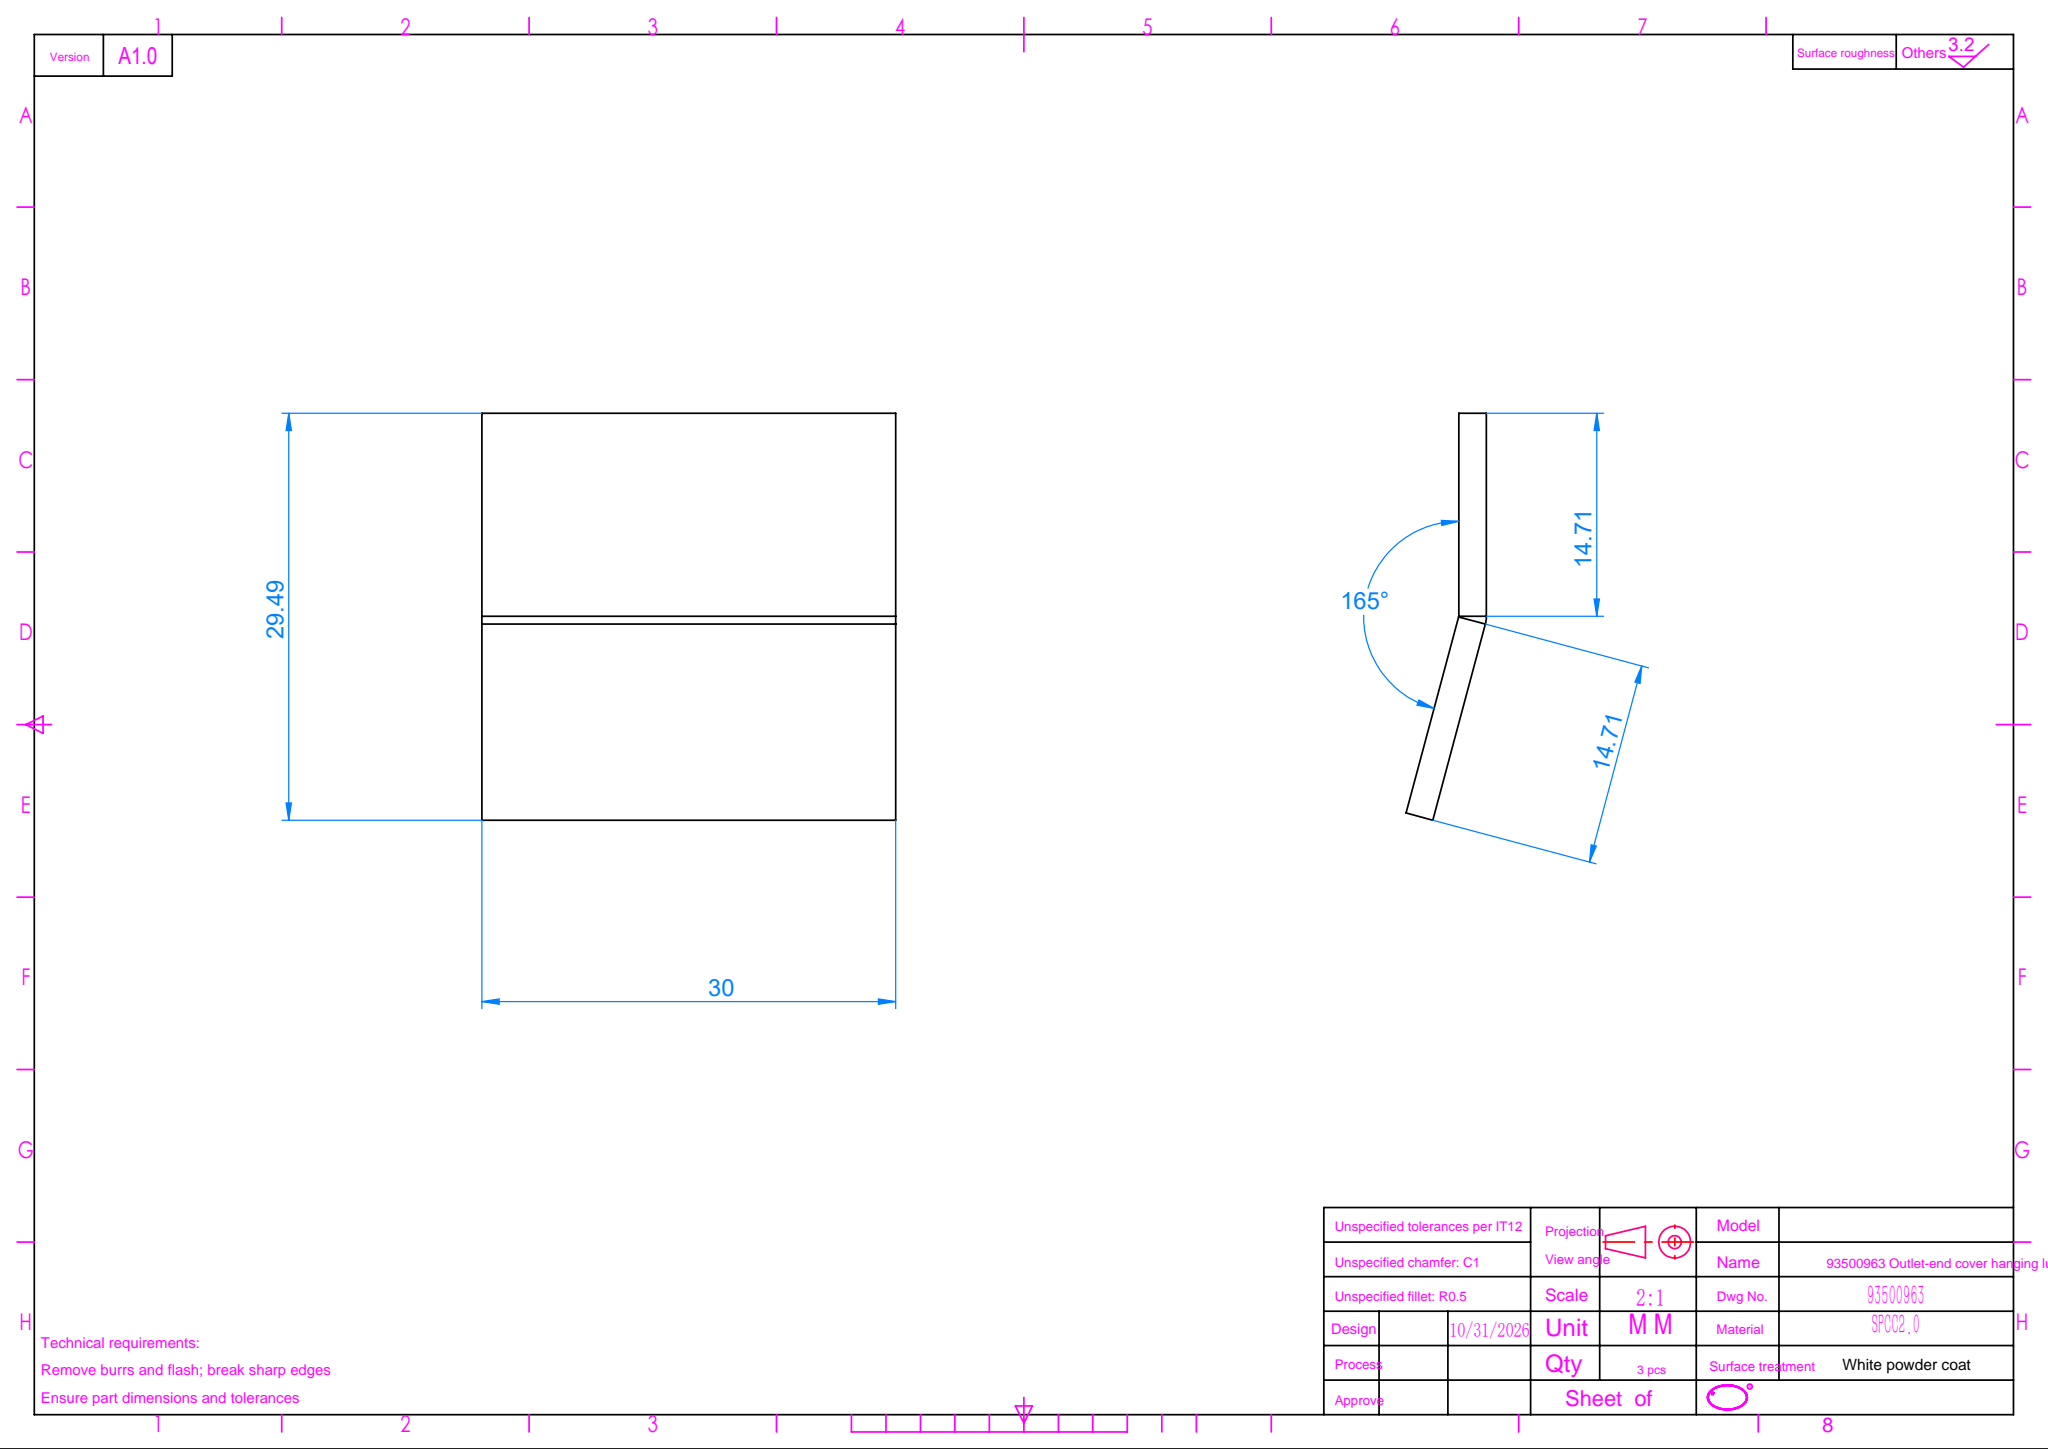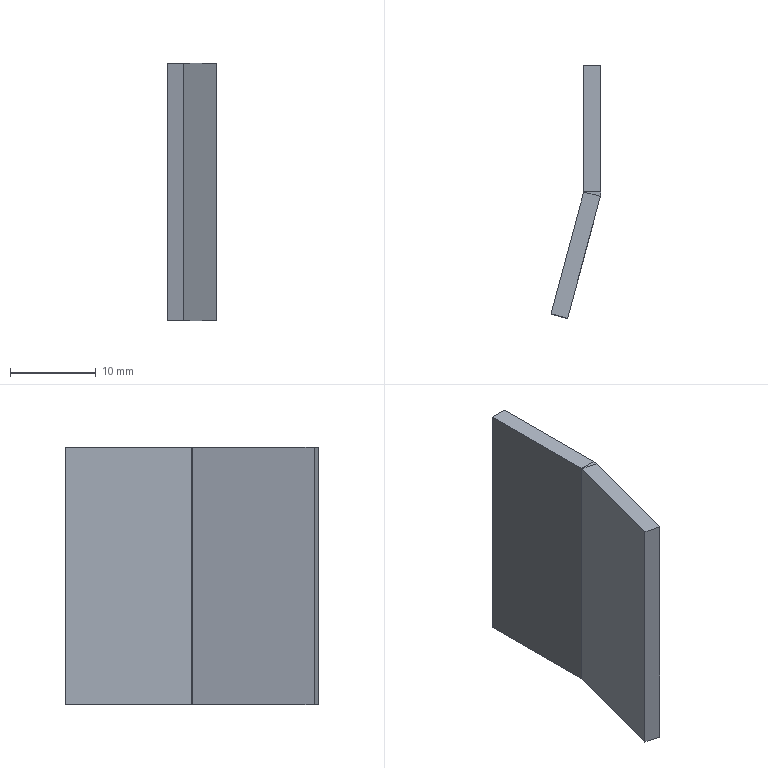Part | SolidWorks | features FlatPattern 1, SMBaseFlange 1, SheetMetal 1 | 1 solid | 14 faces | box 5.814 x 29.489 x 30 mm | volume 1784 mm3 | plane 12 | cylinder 2 | commonest cylinder face diameters 0.4 x1 4.4 x1
STEP:
#1=CARTESIAN_POINT('',(-7.902,11.304,15.));
#2=VERTEX_POINT('',#1);
#3=CARTESIAN_POINT('',(-9.834,11.822,15.));
#4=VERTEX_POINT('',#3);
#5=CARTESIAN_POINT('',(-7.902,11.304,15.));
#6=DIRECTION('',(-0.9659,0.2588,0.));
#7=VECTOR('',#6,1000.);
#8=LINE('',#5,#7);
#9=EDGE_CURVE('',#2,#4,#8,.T.);
#10=ORIENTED_EDGE('',*,*,#9,.F.);
#11=CARTESIAN_POINT('',(-7.827,11.874,15.));
#12=VERTEX_POINT('',#11);
#13=CARTESIAN_POINT('',(-10.027,11.874,15.));
#14=DIRECTION('',(0.,0.,-1.));
#15=DIRECTION('',(1.,0.,0.));
#16=AXIS2_PLACEMENT_3D('',#13,#14,#15);
#17=CIRCLE('',#16,2.2);
#18=EDGE_CURVE('',#12,#2,#17,.T.);
#19=ORIENTED_EDGE('',*,*,#18,.F.);
#20=CARTESIAN_POINT('',(-9.827,11.874,15.));
#21=VERTEX_POINT('',#20);
#22=CARTESIAN_POINT('',(-9.827,11.874,15.));
#23=DIRECTION('',(1.,0.,0.));
#24=VECTOR('',#23,1000.);
#25=LINE('',#22,#24);
#26=EDGE_CURVE('',#21,#12,#25,.T.);
#27=ORIENTED_EDGE('',*,*,#26,.F.);
#28=CARTESIAN_POINT('',(-10.027,11.874,15.));
#29=DIRECTION('',(0.,0.,-1.));
#30=DIRECTION('',(1.,0.,0.));
#31=AXIS2_PLACEMENT_3D('',#28,#29,#30);
#32=CIRCLE('',#31,0.2);
#33=EDGE_CURVE('',#21,#4,#32,.T.);
#34=ORIENTED_EDGE('',*,*,#33,.T.);
#35=EDGE_LOOP('',(#10,#19,#27,#34));
#36=FACE_OUTER_BOUND('',#35,.T.);
#37=CARTESIAN_POINT('',(-7.902,11.304,15.));
#38=DIRECTION('',(0.,0.,1.));
#39=DIRECTION('',(1.,0.,0.));
#40=AXIS2_PLACEMENT_3D('',#37,#38,#39);
#41=PLANE('',#40);
#42=ADVANCED_FACE('',(#36),#41,.T.);
#43=CARTESIAN_POINT('',(-11.71,-2.905,15.));
#44=VERTEX_POINT('',#43);
#45=CARTESIAN_POINT('',(-7.827,11.584,15.));
#46=DIRECTION('',(-0.2588,-0.9659,0.));
#47=VECTOR('',#46,1000.);
#48=LINE('',#45,#47);
#49=EDGE_CURVE('',#2,#44,#48,.T.);
#50=ORIENTED_EDGE('',*,*,#49,.F.);
#51=ORIENTED_EDGE('',*,*,#9,.T.);
#52=CARTESIAN_POINT('',(-13.642,-2.387,15.));
#53=VERTEX_POINT('',#52);
#54=CARTESIAN_POINT('',(-9.759,12.102,15.));
#55=DIRECTION('',(-0.2588,-0.9659,0.));
#56=VECTOR('',#55,1000.);
#57=LINE('',#54,#56);
#58=EDGE_CURVE('',#4,#53,#57,.T.);
#59=ORIENTED_EDGE('',*,*,#58,.T.);
#60=CARTESIAN_POINT('',(-11.71,-2.905,15.));
#61=DIRECTION('',(-0.9659,0.2588,0.));
#62=VECTOR('',#61,1000.);
#63=LINE('',#60,#62);
#64=EDGE_CURVE('',#44,#53,#63,.T.);
#65=ORIENTED_EDGE('',*,*,#64,.F.);
#66=EDGE_LOOP('',(#50,#51,#59,#65));
#67=FACE_OUTER_BOUND('',#66,.T.);
#68=CARTESIAN_POINT('',(-9.827,11.874,15.));
#69=DIRECTION('',(0.,0.,1.));
#70=DIRECTION('',(1.,0.,0.));
#71=AXIS2_PLACEMENT_3D('',#68,#69,#70);
#72=PLANE('',#71);
#73=ADVANCED_FACE('',(#67),#72,.T.);
#74=CARTESIAN_POINT('',(-7.827,11.874,-15.));
#75=VERTEX_POINT('',#74);
#76=CARTESIAN_POINT('',(-9.827,11.874,-15.));
#77=VERTEX_POINT('',#76);
#78=CARTESIAN_POINT('',(-7.827,11.874,-15.));
#79=DIRECTION('',(-1.,0.,0.));
#80=VECTOR('',#79,1000.);
#81=LINE('',#78,#80);
#82=EDGE_CURVE('',#75,#77,#81,.T.);
#83=ORIENTED_EDGE('',*,*,#82,.F.);
#84=CARTESIAN_POINT('',(-7.902,11.304,-15.));
#85=VERTEX_POINT('',#84);
#86=CARTESIAN_POINT('',(-10.027,11.874,-15.));
#87=DIRECTION('',(0.,0.,-1.));
#88=DIRECTION('',(1.,0.,0.));
#89=AXIS2_PLACEMENT_3D('',#86,#87,#88);
#90=CIRCLE('',#89,2.2);
#91=EDGE_CURVE('',#75,#85,#90,.T.);
#92=ORIENTED_EDGE('',*,*,#91,.T.);
#93=CARTESIAN_POINT('',(-9.834,11.822,-15.));
#94=VERTEX_POINT('',#93);
#95=CARTESIAN_POINT('',(-9.834,11.822,-15.));
#96=DIRECTION('',(0.9659,-0.2588,0.));
#97=VECTOR('',#96,1000.);
#98=LINE('',#95,#97);
#99=EDGE_CURVE('',#94,#85,#98,.T.);
#100=ORIENTED_EDGE('',*,*,#99,.F.);
#101=CARTESIAN_POINT('',(-10.027,11.874,-15.));
#102=DIRECTION('',(0.,0.,-1.));
#103=DIRECTION('',(1.,0.,0.));
#104=AXIS2_PLACEMENT_3D('',#101,#102,#103);
#105=CIRCLE('',#104,0.2);
#106=EDGE_CURVE('',#77,#94,#105,.T.);
#107=ORIENTED_EDGE('',*,*,#106,.F.);
#108=EDGE_LOOP('',(#83,#92,#100,#107));
#109=FACE_OUTER_BOUND('',#108,.T.);
#110=CARTESIAN_POINT('',(-7.827,11.874,-15.));
#111=DIRECTION('',(0.,0.,-1.));
#112=DIRECTION('',(-1.,0.,0.));
#113=AXIS2_PLACEMENT_3D('',#110,#111,#112);
#114=PLANE('',#113);
#115=ADVANCED_FACE('',(#109),#114,.T.);
#116=CARTESIAN_POINT('',(-7.827,26.584,-15.));
#117=VERTEX_POINT('',#116);
#118=CARTESIAN_POINT('',(-7.827,26.584,-15.));
#119=DIRECTION('',(0.,-1.,0.));
#120=VECTOR('',#119,1000.);
#121=LINE('',#118,#120);
#122=EDGE_CURVE('',#117,#75,#121,.T.);
#123=ORIENTED_EDGE('',*,*,#122,.T.);
#124=ORIENTED_EDGE('',*,*,#82,.T.);
#125=CARTESIAN_POINT('',(-9.827,26.584,-15.));
#126=VERTEX_POINT('',#125);
#127=CARTESIAN_POINT('',(-9.827,26.584,-15.));
#128=DIRECTION('',(0.,-1.,0.));
#129=VECTOR('',#128,1000.);
#130=LINE('',#127,#129);
#131=EDGE_CURVE('',#126,#77,#130,.T.);
#132=ORIENTED_EDGE('',*,*,#131,.F.);
#133=CARTESIAN_POINT('',(-9.827,26.584,-15.));
#134=DIRECTION('',(1.,0.,0.));
#135=VECTOR('',#134,1000.);
#136=LINE('',#133,#135);
#137=EDGE_CURVE('',#126,#117,#136,.T.);
#138=ORIENTED_EDGE('',*,*,#137,.T.);
#139=EDGE_LOOP('',(#123,#124,#132,#138));
#140=FACE_OUTER_BOUND('',#139,.T.);
#141=CARTESIAN_POINT('',(-9.834,11.822,-15.));
#142=DIRECTION('',(0.,0.,-1.));
#143=DIRECTION('',(-1.,0.,0.));
#144=AXIS2_PLACEMENT_3D('',#141,#142,#143);
#145=PLANE('',#144);
#146=ADVANCED_FACE('',(#140),#145,.T.);
#147=CARTESIAN_POINT('',(-9.834,11.822,15.));
#148=DIRECTION('',(0.,0.,-1.));
#149=VECTOR('',#148,1000.);
#150=LINE('',#147,#149);
#151=EDGE_CURVE('',#4,#94,#150,.T.);
#152=ORIENTED_EDGE('',*,*,#151,.T.);
#153=CARTESIAN_POINT('',(-13.642,-2.387,-15.));
#154=VERTEX_POINT('',#153);
#155=CARTESIAN_POINT('',(-9.759,12.102,-15.));
#156=DIRECTION('',(-0.2588,-0.9659,0.));
#157=VECTOR('',#156,1000.);
#158=LINE('',#155,#157);
#159=EDGE_CURVE('',#94,#154,#158,.T.);
#160=ORIENTED_EDGE('',*,*,#159,.T.);
#161=CARTESIAN_POINT('',(-13.642,-2.387,15.));
#162=DIRECTION('',(0.,0.,-1.));
#163=VECTOR('',#162,1000.);
#164=LINE('',#161,#163);
#165=EDGE_CURVE('',#53,#154,#164,.T.);
#166=ORIENTED_EDGE('',*,*,#165,.F.);
#167=ORIENTED_EDGE('',*,*,#58,.F.);
#168=EDGE_LOOP('',(#152,#160,#166,#167));
#169=FACE_OUTER_BOUND('',#168,.T.);
#170=CARTESIAN_POINT('',(-9.759,12.102,15.));
#171=DIRECTION('',(0.9659,-0.2588,0.));
#172=DIRECTION('',(0.2588,0.9659,0.));
#173=AXIS2_PLACEMENT_3D('',#170,#171,#172);
#174=PLANE('',#173);
#175=ADVANCED_FACE('',(#169),#174,.F.);
#176=ORIENTED_EDGE('',*,*,#165,.T.);
#177=CARTESIAN_POINT('',(-11.71,-2.905,-15.));
#178=VERTEX_POINT('',#177);
#179=CARTESIAN_POINT('',(-11.71,-2.905,-15.));
#180=DIRECTION('',(-0.9659,0.2588,0.));
#181=VECTOR('',#180,1000.);
#182=LINE('',#179,#181);
#183=EDGE_CURVE('',#178,#154,#182,.T.);
#184=ORIENTED_EDGE('',*,*,#183,.F.);
#185=CARTESIAN_POINT('',(-11.71,-2.905,15.));
#186=DIRECTION('',(0.,0.,-1.));
#187=VECTOR('',#186,1000.);
#188=LINE('',#185,#187);
#189=EDGE_CURVE('',#44,#178,#188,.T.);
#190=ORIENTED_EDGE('',*,*,#189,.F.);
#191=ORIENTED_EDGE('',*,*,#64,.T.);
#192=EDGE_LOOP('',(#176,#184,#190,#191));
#193=FACE_OUTER_BOUND('',#192,.T.);
#194=CARTESIAN_POINT('',(-11.71,-2.905,15.));
#195=DIRECTION('',(-0.2588,-0.9659,0.));
#196=DIRECTION('',(0.9659,-0.2588,0.));
#197=AXIS2_PLACEMENT_3D('',#194,#195,#196);
#198=PLANE('',#197);
#199=ADVANCED_FACE('',(#193),#198,.T.);
#200=ORIENTED_EDGE('',*,*,#189,.T.);
#201=CARTESIAN_POINT('',(-7.827,11.584,-15.));
#202=DIRECTION('',(-0.2588,-0.9659,0.));
#203=VECTOR('',#202,1000.);
#204=LINE('',#201,#203);
#205=EDGE_CURVE('',#85,#178,#204,.T.);
#206=ORIENTED_EDGE('',*,*,#205,.F.);
#207=CARTESIAN_POINT('',(-7.902,11.304,15.));
#208=DIRECTION('',(0.,0.,-1.));
#209=VECTOR('',#208,1000.);
#210=LINE('',#207,#209);
#211=EDGE_CURVE('',#2,#85,#210,.T.);
#212=ORIENTED_EDGE('',*,*,#211,.F.);
#213=ORIENTED_EDGE('',*,*,#49,.T.);
#214=EDGE_LOOP('',(#200,#206,#212,#213));
#215=FACE_OUTER_BOUND('',#214,.T.);
#216=CARTESIAN_POINT('',(-7.827,11.584,15.));
#217=DIRECTION('',(0.9659,-0.2588,0.));
#218=DIRECTION('',(0.2588,0.9659,0.));
#219=AXIS2_PLACEMENT_3D('',#216,#217,#218);
#220=PLANE('',#219);
#221=ADVANCED_FACE('',(#215),#220,.T.);
#222=ORIENTED_EDGE('',*,*,#211,.T.);
#223=ORIENTED_EDGE('',*,*,#91,.F.);
#224=CARTESIAN_POINT('',(-7.827,11.874,15.));
#225=DIRECTION('',(0.,0.,-1.));
#226=VECTOR('',#225,1000.);
#227=LINE('',#224,#226);
#228=EDGE_CURVE('',#12,#75,#227,.T.);
#229=ORIENTED_EDGE('',*,*,#228,.F.);
#230=ORIENTED_EDGE('',*,*,#18,.T.);
#231=EDGE_LOOP('',(#222,#223,#229,#230));
#232=FACE_OUTER_BOUND('',#231,.T.);
#233=CARTESIAN_POINT('',(-10.027,11.874,15.));
#234=DIRECTION('',(0.,0.,-1.));
#235=DIRECTION('',(-1.,0.,0.));
#236=AXIS2_PLACEMENT_3D('',#233,#234,#235);
#237=CYLINDRICAL_SURFACE('',#236,2.2);
#238=ADVANCED_FACE('',(#232),#237,.T.);
#239=ORIENTED_EDGE('',*,*,#228,.T.);
#240=ORIENTED_EDGE('',*,*,#122,.F.);
#241=CARTESIAN_POINT('',(-7.827,26.584,15.));
#242=VERTEX_POINT('',#241);
#243=CARTESIAN_POINT('',(-7.827,26.584,15.));
#244=DIRECTION('',(0.,0.,-1.));
#245=VECTOR('',#244,1000.);
#246=LINE('',#243,#245);
#247=EDGE_CURVE('',#242,#117,#246,.T.);
#248=ORIENTED_EDGE('',*,*,#247,.F.);
#249=CARTESIAN_POINT('',(-7.827,26.584,15.));
#250=DIRECTION('',(0.,-1.,0.));
#251=VECTOR('',#250,1000.);
#252=LINE('',#249,#251);
#253=EDGE_CURVE('',#242,#12,#252,.T.);
#254=ORIENTED_EDGE('',*,*,#253,.T.);
#255=EDGE_LOOP('',(#239,#240,#248,#254));
#256=FACE_OUTER_BOUND('',#255,.T.);
#257=CARTESIAN_POINT('',(-7.827,26.584,15.));
#258=DIRECTION('',(1.,0.,0.));
#259=DIRECTION('',(0.,1.,0.));
#260=AXIS2_PLACEMENT_3D('',#257,#258,#259);
#261=PLANE('',#260);
#262=ADVANCED_FACE('',(#256),#261,.T.);
#263=ORIENTED_EDGE('',*,*,#247,.T.);
#264=ORIENTED_EDGE('',*,*,#137,.F.);
#265=CARTESIAN_POINT('',(-9.827,26.584,15.));
#266=VERTEX_POINT('',#265);
#267=CARTESIAN_POINT('',(-9.827,26.584,15.));
#268=DIRECTION('',(0.,0.,-1.));
#269=VECTOR('',#268,1000.);
#270=LINE('',#267,#269);
#271=EDGE_CURVE('',#266,#126,#270,.T.);
#272=ORIENTED_EDGE('',*,*,#271,.F.);
#273=CARTESIAN_POINT('',(-9.827,26.584,15.));
#274=DIRECTION('',(1.,0.,0.));
#275=VECTOR('',#274,1000.);
#276=LINE('',#273,#275);
#277=EDGE_CURVE('',#266,#242,#276,.T.);
#278=ORIENTED_EDGE('',*,*,#277,.T.);
#279=EDGE_LOOP('',(#263,#264,#272,#278));
#280=FACE_OUTER_BOUND('',#279,.T.);
#281=CARTESIAN_POINT('',(-9.827,26.584,15.));
#282=DIRECTION('',(0.,1.,0.));
#283=DIRECTION('',(0.,0.,1.));
#284=AXIS2_PLACEMENT_3D('',#281,#282,#283);
#285=PLANE('',#284);
#286=ADVANCED_FACE('',(#280),#285,.T.);
#287=ORIENTED_EDGE('',*,*,#271,.T.);
#288=ORIENTED_EDGE('',*,*,#131,.T.);
#289=CARTESIAN_POINT('',(-9.827,11.874,15.));
#290=DIRECTION('',(0.,0.,-1.));
#291=VECTOR('',#290,1000.);
#292=LINE('',#289,#291);
#293=EDGE_CURVE('',#21,#77,#292,.T.);
#294=ORIENTED_EDGE('',*,*,#293,.F.);
#295=CARTESIAN_POINT('',(-9.827,26.584,15.));
#296=DIRECTION('',(0.,-1.,0.));
#297=VECTOR('',#296,1000.);
#298=LINE('',#295,#297);
#299=EDGE_CURVE('',#266,#21,#298,.T.);
#300=ORIENTED_EDGE('',*,*,#299,.F.);
#301=EDGE_LOOP('',(#287,#288,#294,#300));
#302=FACE_OUTER_BOUND('',#301,.T.);
#303=CARTESIAN_POINT('',(-9.827,26.584,15.));
#304=DIRECTION('',(1.,0.,0.));
#305=DIRECTION('',(0.,1.,0.));
#306=AXIS2_PLACEMENT_3D('',#303,#304,#305);
#307=PLANE('',#306);
#308=ADVANCED_FACE('',(#302),#307,.F.);
#309=ORIENTED_EDGE('',*,*,#293,.T.);
#310=ORIENTED_EDGE('',*,*,#106,.T.);
#311=ORIENTED_EDGE('',*,*,#151,.F.);
#312=ORIENTED_EDGE('',*,*,#33,.F.);
#313=EDGE_LOOP('',(#309,#310,#311,#312));
#314=FACE_OUTER_BOUND('',#313,.T.);
#315=CARTESIAN_POINT('',(-10.027,11.874,15.));
#316=DIRECTION('',(0.,0.,-1.));
#317=DIRECTION('',(-1.,0.,0.));
#318=AXIS2_PLACEMENT_3D('',#315,#316,#317);
#319=CYLINDRICAL_SURFACE('',#318,0.2);
#320=ADVANCED_FACE('',(#314),#319,.F.);
#321=ORIENTED_EDGE('',*,*,#299,.T.);
#322=ORIENTED_EDGE('',*,*,#26,.T.);
#323=ORIENTED_EDGE('',*,*,#253,.F.);
#324=ORIENTED_EDGE('',*,*,#277,.F.);
#325=EDGE_LOOP('',(#321,#322,#323,#324));
#326=FACE_OUTER_BOUND('',#325,.T.);
#327=CARTESIAN_POINT('',(-10.027,11.874,15.));
#328=DIRECTION('',(0.,0.,1.));
#329=DIRECTION('',(1.,0.,0.));
#330=AXIS2_PLACEMENT_3D('',#327,#328,#329);
#331=PLANE('',#330);
#332=ADVANCED_FACE('',(#326),#331,.T.);
#333=ORIENTED_EDGE('',*,*,#159,.F.);
#334=ORIENTED_EDGE('',*,*,#99,.T.);
#335=ORIENTED_EDGE('',*,*,#205,.T.);
#336=ORIENTED_EDGE('',*,*,#183,.T.);
#337=EDGE_LOOP('',(#333,#334,#335,#336));
#338=FACE_OUTER_BOUND('',#337,.T.);
#339=CARTESIAN_POINT('',(-10.027,11.874,-15.));
#340=DIRECTION('',(0.,0.,1.));
#341=DIRECTION('',(1.,0.,0.));
#342=AXIS2_PLACEMENT_3D('',#339,#340,#341);
#343=PLANE('',#342);
#344=ADVANCED_FACE('',(#338),#343,.F.);
#345=CLOSED_SHELL('',(#42,#73,#115,#146,#175,#199,#221,#238,#262,#286,#308,#320,#332,#344));
#346=MANIFOLD_SOLID_BREP('',#345);
#347=CARTESIAN_POINT('',(0.,0.,0.));
#348=DIRECTION('',(0.,0.,1.));
#349=DIRECTION('',(1.,0.,0.));
#350=AXIS2_PLACEMENT_3D('',#347,#348,#349);
#351=(LENGTH_UNIT()NAMED_UNIT(*)SI_UNIT(.MILLI.,.METRE.));
#352=UNCERTAINTY_MEASURE_WITH_UNIT(LENGTH_MEASURE(0.00001),#351,'','');
#353=(NAMED_UNIT(*)PLANE_ANGLE_UNIT()SI_UNIT($,.RADIAN.));
#354=(NAMED_UNIT(*)SI_UNIT($,.STERADIAN.)SOLID_ANGLE_UNIT());
#355=(GEOMETRIC_REPRESENTATION_CONTEXT(3)GLOBAL_UNCERTAINTY_ASSIGNED_CONTEXT((#352))GLOBAL_UNIT_ASSIGNED_CONTEXT((#351,#353,#354))REPRESENTATION_CONTEXT('',''));
#356=ADVANCED_BREP_SHAPE_REPRESENTATION('',(#346,#350),#355);